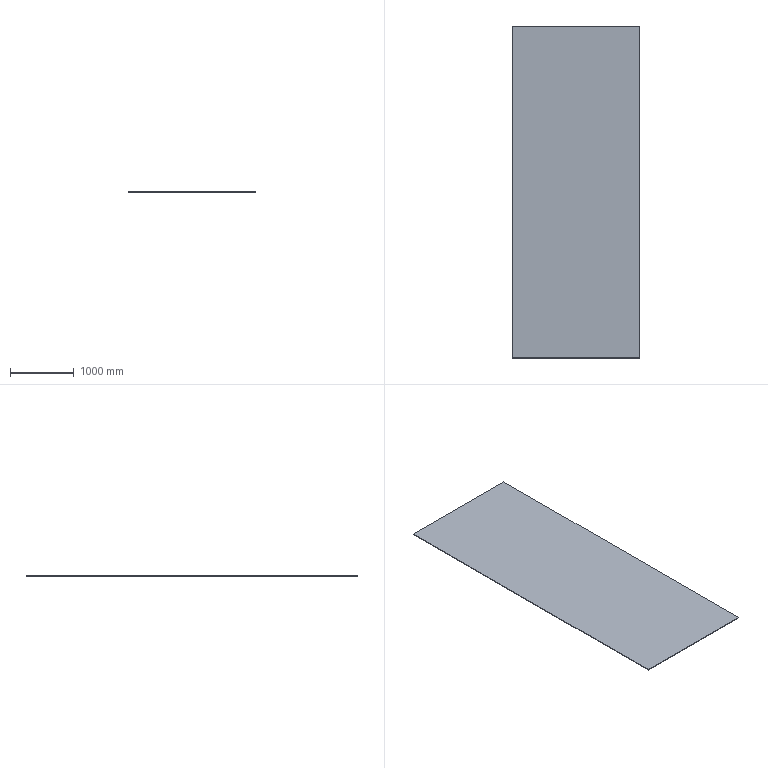Part | Creo | features DATUM PLANE 3, COORDINATE SYSTEM 1, CURVE 1, PROTRUSION 1 | 1 solid | 6 faces | box 2000 x 5200 x 10 mm | volume 104000000 mm3 | plane 6
STEP:
#1=CARTESIAN_POINT('',(0.,0.,0.));
#2=DIRECTION('',(0.,0.,1.));
#3=DIRECTION('',(1.,0.,0.));
#4=AXIS2_PLACEMENT_3D('',#1,#2,#3);
#5=CARTESIAN_POINT('',(1000.,-2600.,0.));
#6=VERTEX_POINT('',#5);
#7=CARTESIAN_POINT('',(1000.,2600.,0.));
#8=VERTEX_POINT('',#7);
#9=CARTESIAN_POINT('',(1000.,-2600.,0.));
#10=DIRECTION('',(0.,1.,0.));
#11=VECTOR('',#10,5200.);
#12=LINE('',#9,#11);
#13=EDGE_CURVE('',#6,#8,#12,.T.);
#14=ORIENTED_EDGE('',*,*,#13,.T.);
#15=CARTESIAN_POINT('',(-1000.,2600.,0.));
#16=VERTEX_POINT('',#15);
#17=CARTESIAN_POINT('',(1000.,2600.,0.));
#18=DIRECTION('',(-1.,0.,0.));
#19=VECTOR('',#18,2000.);
#20=LINE('',#17,#19);
#21=EDGE_CURVE('',#8,#16,#20,.T.);
#22=ORIENTED_EDGE('',*,*,#21,.T.);
#23=CARTESIAN_POINT('',(-1000.,-2600.,0.));
#24=VERTEX_POINT('',#23);
#25=CARTESIAN_POINT('',(-1000.,2600.,0.));
#26=DIRECTION('',(0.,-1.,0.));
#27=VECTOR('',#26,5200.);
#28=LINE('',#25,#27);
#29=EDGE_CURVE('',#16,#24,#28,.T.);
#30=ORIENTED_EDGE('',*,*,#29,.T.);
#31=CARTESIAN_POINT('',(-1000.,-2600.,0.));
#32=DIRECTION('',(1.,0.,0.));
#33=VECTOR('',#32,2000.);
#34=LINE('',#31,#33);
#35=EDGE_CURVE('',#24,#6,#34,.T.);
#36=ORIENTED_EDGE('',*,*,#35,.T.);
#37=EDGE_LOOP('',(#14,#22,#30,#36));
#38=FACE_OUTER_BOUND('',#37,.F.);
#39=CARTESIAN_POINT('',(0.,0.,0.));
#40=DIRECTION('',(0.,0.,1.));
#41=DIRECTION('',(1.,0.,0.));
#42=AXIS2_PLACEMENT_3D('',#39,#40,#41);
#43=PLANE('',#42);
#44=ADVANCED_FACE('',(#38),#43,.F.);
#45=ORIENTED_EDGE('',*,*,#13,.F.);
#46=CARTESIAN_POINT('',(1000.,-2600.,10.));
#47=VERTEX_POINT('',#46);
#48=CARTESIAN_POINT('',(1000.,-2600.,0.));
#49=DIRECTION('',(0.,0.,1.));
#50=VECTOR('',#49,10.);
#51=LINE('',#48,#50);
#52=EDGE_CURVE('',#6,#47,#51,.T.);
#53=ORIENTED_EDGE('',*,*,#52,.T.);
#54=CARTESIAN_POINT('',(1000.,2600.,10.));
#55=VERTEX_POINT('',#54);
#56=CARTESIAN_POINT('',(1000.,-2600.,10.));
#57=DIRECTION('',(0.,1.,0.));
#58=VECTOR('',#57,5200.);
#59=LINE('',#56,#58);
#60=EDGE_CURVE('',#47,#55,#59,.T.);
#61=ORIENTED_EDGE('',*,*,#60,.T.);
#62=CARTESIAN_POINT('',(1000.,2600.,0.));
#63=DIRECTION('',(0.,0.,1.));
#64=VECTOR('',#63,10.);
#65=LINE('',#62,#64);
#66=EDGE_CURVE('',#8,#55,#65,.T.);
#67=ORIENTED_EDGE('',*,*,#66,.F.);
#68=EDGE_LOOP('',(#45,#53,#61,#67));
#69=FACE_OUTER_BOUND('',#68,.F.);
#70=CARTESIAN_POINT('',(1000.,-2600.,0.));
#71=DIRECTION('',(1.,0.,0.));
#72=DIRECTION('',(0.,1.,0.));
#73=AXIS2_PLACEMENT_3D('',#70,#71,#72);
#74=PLANE('',#73);
#75=ADVANCED_FACE('',(#69),#74,.T.);
#76=ORIENTED_EDGE('',*,*,#35,.F.);
#77=CARTESIAN_POINT('',(-1000.,-2600.,10.));
#78=VERTEX_POINT('',#77);
#79=CARTESIAN_POINT('',(-1000.,-2600.,0.));
#80=DIRECTION('',(0.,0.,1.));
#81=VECTOR('',#80,10.);
#82=LINE('',#79,#81);
#83=EDGE_CURVE('',#24,#78,#82,.T.);
#84=ORIENTED_EDGE('',*,*,#83,.T.);
#85=CARTESIAN_POINT('',(-1000.,-2600.,10.));
#86=DIRECTION('',(1.,0.,0.));
#87=VECTOR('',#86,2000.);
#88=LINE('',#85,#87);
#89=EDGE_CURVE('',#78,#47,#88,.T.);
#90=ORIENTED_EDGE('',*,*,#89,.T.);
#91=ORIENTED_EDGE('',*,*,#52,.F.);
#92=EDGE_LOOP('',(#76,#84,#90,#91));
#93=FACE_OUTER_BOUND('',#92,.F.);
#94=CARTESIAN_POINT('',(-1000.,-2600.,0.));
#95=DIRECTION('',(0.,-1.,0.));
#96=DIRECTION('',(1.,0.,0.));
#97=AXIS2_PLACEMENT_3D('',#94,#95,#96);
#98=PLANE('',#97);
#99=ADVANCED_FACE('',(#93),#98,.T.);
#100=ORIENTED_EDGE('',*,*,#29,.F.);
#101=CARTESIAN_POINT('',(-1000.,2600.,10.));
#102=VERTEX_POINT('',#101);
#103=CARTESIAN_POINT('',(-1000.,2600.,0.));
#104=DIRECTION('',(0.,0.,1.));
#105=VECTOR('',#104,10.);
#106=LINE('',#103,#105);
#107=EDGE_CURVE('',#16,#102,#106,.T.);
#108=ORIENTED_EDGE('',*,*,#107,.T.);
#109=CARTESIAN_POINT('',(-1000.,2600.,10.));
#110=DIRECTION('',(0.,-1.,0.));
#111=VECTOR('',#110,5200.);
#112=LINE('',#109,#111);
#113=EDGE_CURVE('',#102,#78,#112,.T.);
#114=ORIENTED_EDGE('',*,*,#113,.T.);
#115=ORIENTED_EDGE('',*,*,#83,.F.);
#116=EDGE_LOOP('',(#100,#108,#114,#115));
#117=FACE_OUTER_BOUND('',#116,.F.);
#118=CARTESIAN_POINT('',(-1000.,2600.,0.));
#119=DIRECTION('',(-1.,0.,0.));
#120=DIRECTION('',(0.,-1.,0.));
#121=AXIS2_PLACEMENT_3D('',#118,#119,#120);
#122=PLANE('',#121);
#123=ADVANCED_FACE('',(#117),#122,.T.);
#124=ORIENTED_EDGE('',*,*,#21,.F.);
#125=ORIENTED_EDGE('',*,*,#66,.T.);
#126=CARTESIAN_POINT('',(1000.,2600.,10.));
#127=DIRECTION('',(-1.,0.,0.));
#128=VECTOR('',#127,2000.);
#129=LINE('',#126,#128);
#130=EDGE_CURVE('',#55,#102,#129,.T.);
#131=ORIENTED_EDGE('',*,*,#130,.T.);
#132=ORIENTED_EDGE('',*,*,#107,.F.);
#133=EDGE_LOOP('',(#124,#125,#131,#132));
#134=FACE_OUTER_BOUND('',#133,.F.);
#135=CARTESIAN_POINT('',(1000.,2600.,0.));
#136=DIRECTION('',(0.,1.,0.));
#137=DIRECTION('',(-1.,0.,0.));
#138=AXIS2_PLACEMENT_3D('',#135,#136,#137);
#139=PLANE('',#138);
#140=ADVANCED_FACE('',(#134),#139,.T.);
#141=ORIENTED_EDGE('',*,*,#60,.F.);
#142=ORIENTED_EDGE('',*,*,#89,.F.);
#143=ORIENTED_EDGE('',*,*,#113,.F.);
#144=ORIENTED_EDGE('',*,*,#130,.F.);
#145=EDGE_LOOP('',(#141,#142,#143,#144));
#146=FACE_OUTER_BOUND('',#145,.F.);
#147=CARTESIAN_POINT('',(0.,0.,10.));
#148=DIRECTION('',(0.,0.,1.));
#149=DIRECTION('',(1.,0.,0.));
#150=AXIS2_PLACEMENT_3D('',#147,#148,#149);
#151=PLANE('',#150);
#152=ADVANCED_FACE('',(#146),#151,.T.);
#153=CLOSED_SHELL('',(#44,#75,#99,#123,#140,#152));
#154=MANIFOLD_SOLID_BREP('',#153);
#155=(LENGTH_UNIT()NAMED_UNIT(*)SI_UNIT(.MILLI.,.METRE.));
#156=UNCERTAINTY_MEASURE_WITH_UNIT(LENGTH_MEASURE(0.5571),#155,'','');
#157=(NAMED_UNIT(*)PLANE_ANGLE_UNIT()SI_UNIT($,.RADIAN.));
#158=PLANE_ANGLE_MEASURE_WITH_UNIT(PLANE_ANGLE_MEASURE(0.01745),#157);
#159=(CONVERSION_BASED_UNIT('DEGREE',#158)NAMED_UNIT(*)PLANE_ANGLE_UNIT());
#160=(NAMED_UNIT(*)SI_UNIT($,.STERADIAN.)SOLID_ANGLE_UNIT());
#161=(GEOMETRIC_REPRESENTATION_CONTEXT(3)GLOBAL_UNCERTAINTY_ASSIGNED_CONTEXT((#156))GLOBAL_UNIT_ASSIGNED_CONTEXT((#155,#159,#160))REPRESENTATION_CONTEXT('',''));
#162=ADVANCED_BREP_SHAPE_REPRESENTATION('',(#4,#154),#161);